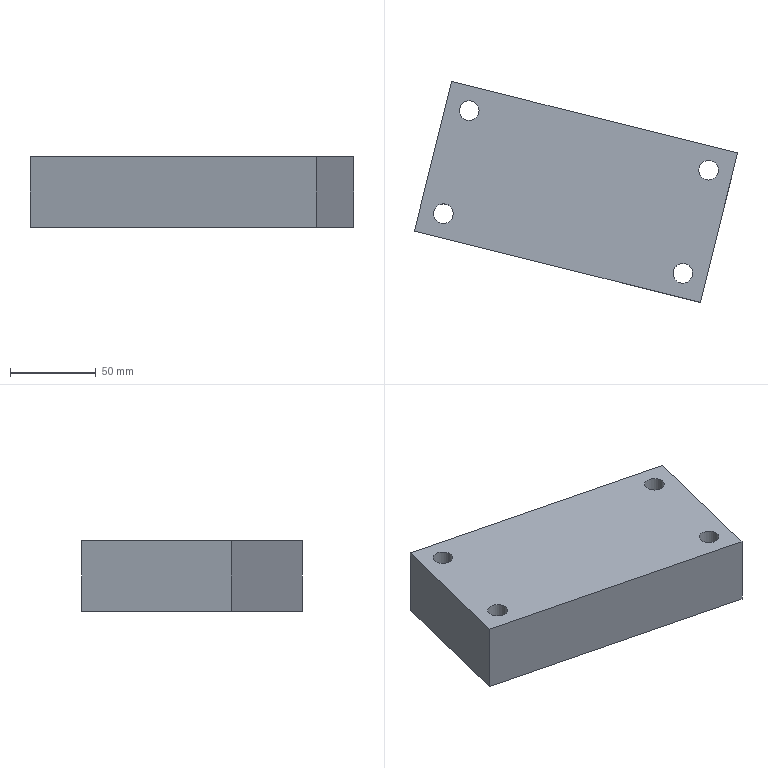Part | NX | features solid 2 | 1 solid | 18 faces | box 188.664 x 128.937 x 41 mm | volume 609814 mm3 | plane 10 | cylinder 8 | commonest cylinder face diameters 11.5 x4 18 x4
STEP:
#1=CARTESIAN_POINT('',(1088.08,30.743,73.));
#2=VERTEX_POINT('',#1);
#3=CARTESIAN_POINT('',(1086.688,25.164,73.));
#4=DIRECTION('',(0.,0.,-1.));
#5=DIRECTION('',(0.2419,0.9703,0.));
#6=AXIS2_PLACEMENT_3D('',#3,#4,#5);
#7=CIRCLE('',#6,5.75);
#8=EDGE_CURVE('',#2,#2,#7,.T.);
#9=ORIENTED_EDGE('',*,*,#8,.F.);
#10=EDGE_LOOP('',(#9));
#11=FACE_BOUND('',#10,.T.);
#12=CARTESIAN_POINT('',(1088.866,33.896,73.));
#13=VERTEX_POINT('',#12);
#14=CARTESIAN_POINT('',(1086.688,25.164,73.));
#15=DIRECTION('',(0.,0.,-1.));
#16=DIRECTION('',(0.2419,0.9703,0.));
#17=AXIS2_PLACEMENT_3D('',#14,#15,#16);
#18=CIRCLE('',#17,9.);
#19=EDGE_CURVE('',#13,#13,#18,.T.);
#20=ORIENTED_EDGE('',*,*,#19,.T.);
#21=EDGE_LOOP('',(#20));
#22=FACE_BOUND('',#21,.T.);
#23=CARTESIAN_POINT('',(1086.688,25.164,73.));
#24=DIRECTION('',(0.,0.,1.));
#25=DIRECTION('',(-0.2419,-0.9703,0.));
#26=AXIS2_PLACEMENT_3D('',#23,#24,#25);
#27=PLANE('',#26);
#28=ADVANCED_FACE('',(#11,#22),#27,.F.);
#29=CARTESIAN_POINT('',(1103.079,90.901,73.));
#30=VERTEX_POINT('',#29);
#31=CARTESIAN_POINT('',(1101.688,85.322,73.));
#32=DIRECTION('',(0.,0.,-1.));
#33=DIRECTION('',(0.2419,0.9703,0.));
#34=AXIS2_PLACEMENT_3D('',#31,#32,#33);
#35=CIRCLE('',#34,5.75);
#36=EDGE_CURVE('',#30,#30,#35,.T.);
#37=ORIENTED_EDGE('',*,*,#36,.F.);
#38=EDGE_LOOP('',(#37));
#39=FACE_BOUND('',#38,.T.);
#40=CARTESIAN_POINT('',(1103.865,94.055,73.));
#41=VERTEX_POINT('',#40);
#42=CARTESIAN_POINT('',(1101.688,85.322,73.));
#43=DIRECTION('',(0.,0.,-1.));
#44=DIRECTION('',(0.2419,0.9703,0.));
#45=AXIS2_PLACEMENT_3D('',#42,#43,#44);
#46=CIRCLE('',#45,9.);
#47=EDGE_CURVE('',#41,#41,#46,.T.);
#48=ORIENTED_EDGE('',*,*,#47,.T.);
#49=EDGE_LOOP('',(#48));
#50=FACE_BOUND('',#49,.T.);
#51=CARTESIAN_POINT('',(1101.688,85.322,73.));
#52=DIRECTION('',(0.,0.,1.));
#53=DIRECTION('',(-0.2419,-0.9703,0.));
#54=AXIS2_PLACEMENT_3D('',#51,#52,#53);
#55=PLANE('',#54);
#56=ADVANCED_FACE('',(#39,#50),#55,.F.);
#57=CARTESIAN_POINT('',(948.357,65.58,73.));
#58=VERTEX_POINT('',#57);
#59=CARTESIAN_POINT('',(946.966,60.,73.));
#60=DIRECTION('',(0.,0.,-1.));
#61=DIRECTION('',(0.2419,0.9703,0.));
#62=AXIS2_PLACEMENT_3D('',#59,#60,#61);
#63=CIRCLE('',#62,5.75);
#64=EDGE_CURVE('',#58,#58,#63,.T.);
#65=ORIENTED_EDGE('',*,*,#64,.F.);
#66=EDGE_LOOP('',(#65));
#67=FACE_BOUND('',#66,.T.);
#68=CARTESIAN_POINT('',(949.143,68.733,73.));
#69=VERTEX_POINT('',#68);
#70=CARTESIAN_POINT('',(946.966,60.,73.));
#71=DIRECTION('',(0.,0.,-1.));
#72=DIRECTION('',(0.2419,0.9703,0.));
#73=AXIS2_PLACEMENT_3D('',#70,#71,#72);
#74=CIRCLE('',#73,9.);
#75=EDGE_CURVE('',#69,#69,#74,.T.);
#76=ORIENTED_EDGE('',*,*,#75,.T.);
#77=EDGE_LOOP('',(#76));
#78=FACE_BOUND('',#77,.T.);
#79=CARTESIAN_POINT('',(946.966,60.,73.));
#80=DIRECTION('',(0.,0.,1.));
#81=DIRECTION('',(-0.2419,-0.9703,0.));
#82=AXIS2_PLACEMENT_3D('',#79,#80,#81);
#83=PLANE('',#82);
#84=ADVANCED_FACE('',(#67,#78),#83,.F.);
#85=ORIENTED_EDGE('',*,*,#47,.F.);
#86=EDGE_LOOP('',(#85));
#87=FACE_BOUND('',#86,.T.);
#88=CARTESIAN_POINT('',(1103.865,94.055,60.));
#89=VERTEX_POINT('',#88);
#90=CARTESIAN_POINT('',(1101.688,85.322,60.));
#91=DIRECTION('',(0.,0.,-1.));
#92=DIRECTION('',(0.2419,0.9703,0.));
#93=AXIS2_PLACEMENT_3D('',#90,#91,#92);
#94=CIRCLE('',#93,9.);
#95=EDGE_CURVE('',#89,#89,#94,.T.);
#96=ORIENTED_EDGE('',*,*,#95,.T.);
#97=EDGE_LOOP('',(#96));
#98=FACE_BOUND('',#97,.T.);
#99=CARTESIAN_POINT('',(1101.688,85.322,60.));
#100=DIRECTION('',(0.,0.,1.));
#101=DIRECTION('',(-0.2419,-0.9703,0.));
#102=AXIS2_PLACEMENT_3D('',#99,#100,#101);
#103=CYLINDRICAL_SURFACE('',#102,9.);
#104=ADVANCED_FACE('',(#87,#98),#103,.F.);
#105=ORIENTED_EDGE('',*,*,#75,.F.);
#106=EDGE_LOOP('',(#105));
#107=FACE_BOUND('',#106,.T.);
#108=CARTESIAN_POINT('',(949.143,68.733,60.));
#109=VERTEX_POINT('',#108);
#110=CARTESIAN_POINT('',(946.966,60.,60.));
#111=DIRECTION('',(0.,0.,-1.));
#112=DIRECTION('',(0.2419,0.9703,0.));
#113=AXIS2_PLACEMENT_3D('',#110,#111,#112);
#114=CIRCLE('',#113,9.);
#115=EDGE_CURVE('',#109,#109,#114,.T.);
#116=ORIENTED_EDGE('',*,*,#115,.T.);
#117=EDGE_LOOP('',(#116));
#118=FACE_BOUND('',#117,.T.);
#119=CARTESIAN_POINT('',(946.966,60.,60.));
#120=DIRECTION('',(0.,0.,1.));
#121=DIRECTION('',(-0.2419,-0.9703,0.));
#122=AXIS2_PLACEMENT_3D('',#119,#120,#121);
#123=CYLINDRICAL_SURFACE('',#122,9.);
#124=ADVANCED_FACE('',(#107,#118),#123,.F.);
#125=CARTESIAN_POINT('',(1118.659,95.519,101.));
#126=VERTEX_POINT('',#125);
#127=CARTESIAN_POINT('',(951.768,137.13,101.));
#128=VERTEX_POINT('',#127);
#129=CARTESIAN_POINT('',(1045.886,113.663,101.));
#130=DIRECTION('',(-0.9703,0.2419,0.));
#131=VECTOR('',#130,1000.);
#132=LINE('',#129,#131);
#133=EDGE_CURVE('',#126,#128,#132,.T.);
#134=ORIENTED_EDGE('',*,*,#133,.F.);
#135=CARTESIAN_POINT('',(1118.659,95.519,60.));
#136=VERTEX_POINT('',#135);
#137=CARTESIAN_POINT('',(1118.659,95.519,-25.));
#138=DIRECTION('',(0.,0.,1.));
#139=VECTOR('',#138,1000.);
#140=LINE('',#137,#139);
#141=EDGE_CURVE('',#136,#126,#140,.T.);
#142=ORIENTED_EDGE('',*,*,#141,.F.);
#143=CARTESIAN_POINT('',(951.768,137.13,60.));
#144=VERTEX_POINT('',#143);
#145=CARTESIAN_POINT('',(1045.886,113.663,60.));
#146=DIRECTION('',(0.9703,-0.2419,0.));
#147=VECTOR('',#146,1000.);
#148=LINE('',#145,#147);
#149=EDGE_CURVE('',#144,#136,#148,.T.);
#150=ORIENTED_EDGE('',*,*,#149,.F.);
#151=CARTESIAN_POINT('',(951.768,137.13,-25.));
#152=DIRECTION('',(0.,0.,1.));
#153=VECTOR('',#152,1000.);
#154=LINE('',#151,#153);
#155=EDGE_CURVE('',#144,#128,#154,.T.);
#156=ORIENTED_EDGE('',*,*,#155,.T.);
#157=EDGE_LOOP('',(#134,#142,#150,#156));
#158=FACE_BOUND('',#157,.T.);
#159=CARTESIAN_POINT('',(1045.886,113.663,-25.));
#160=DIRECTION('',(0.2419,0.9703,0.));
#161=DIRECTION('',(0.,0.,1.));
#162=AXIS2_PLACEMENT_3D('',#159,#160,#161);
#163=PLANE('',#162);
#164=ADVANCED_FACE('',(#158),#163,.T.);
#165=CARTESIAN_POINT('',(1096.886,8.193,60.));
#166=VERTEX_POINT('',#165);
#167=CARTESIAN_POINT('',(1096.886,8.193,101.));
#168=VERTEX_POINT('',#167);
#169=CARTESIAN_POINT('',(1096.886,8.193,-25.));
#170=DIRECTION('',(0.,0.,1.));
#171=VECTOR('',#170,1000.);
#172=LINE('',#169,#171);
#173=EDGE_CURVE('',#166,#168,#172,.T.);
#174=ORIENTED_EDGE('',*,*,#173,.F.);
#175=CARTESIAN_POINT('',(1107.772,51.856,60.));
#176=DIRECTION('',(-0.2419,-0.9703,0.));
#177=VECTOR('',#176,1000.);
#178=LINE('',#175,#177);
#179=EDGE_CURVE('',#136,#166,#178,.T.);
#180=ORIENTED_EDGE('',*,*,#179,.F.);
#181=ORIENTED_EDGE('',*,*,#141,.T.);
#182=CARTESIAN_POINT('',(1107.772,51.856,101.));
#183=DIRECTION('',(0.2419,0.9703,0.));
#184=VECTOR('',#183,1000.);
#185=LINE('',#182,#184);
#186=EDGE_CURVE('',#168,#126,#185,.T.);
#187=ORIENTED_EDGE('',*,*,#186,.F.);
#188=EDGE_LOOP('',(#174,#180,#181,#187));
#189=FACE_BOUND('',#188,.T.);
#190=CARTESIAN_POINT('',(1107.772,51.856,-25.));
#191=DIRECTION('',(0.9703,-0.2419,0.));
#192=DIRECTION('',(0.,0.,-1.));
#193=AXIS2_PLACEMENT_3D('',#190,#191,#192);
#194=PLANE('',#193);
#195=ADVANCED_FACE('',(#189),#194,.T.);
#196=CARTESIAN_POINT('',(929.995,49.803,60.));
#197=VERTEX_POINT('',#196);
#198=CARTESIAN_POINT('',(929.995,49.803,101.));
#199=VERTEX_POINT('',#198);
#200=CARTESIAN_POINT('',(929.995,49.803,-25.));
#201=DIRECTION('',(0.,0.,1.));
#202=VECTOR('',#201,1000.);
#203=LINE('',#200,#202);
#204=EDGE_CURVE('',#197,#199,#203,.T.);
#205=ORIENTED_EDGE('',*,*,#204,.F.);
#206=CARTESIAN_POINT('',(1024.114,26.337,60.));
#207=DIRECTION('',(-0.9703,0.2419,0.));
#208=VECTOR('',#207,1000.);
#209=LINE('',#206,#208);
#210=EDGE_CURVE('',#166,#197,#209,.T.);
#211=ORIENTED_EDGE('',*,*,#210,.F.);
#212=ORIENTED_EDGE('',*,*,#173,.T.);
#213=CARTESIAN_POINT('',(1024.114,26.337,101.));
#214=DIRECTION('',(0.9703,-0.2419,0.));
#215=VECTOR('',#214,1000.);
#216=LINE('',#213,#215);
#217=EDGE_CURVE('',#199,#168,#216,.T.);
#218=ORIENTED_EDGE('',*,*,#217,.F.);
#219=EDGE_LOOP('',(#205,#211,#212,#218));
#220=FACE_BOUND('',#219,.T.);
#221=CARTESIAN_POINT('',(1024.114,26.337,-25.));
#222=DIRECTION('',(-0.2419,-0.9703,0.));
#223=DIRECTION('',(0.,0.,-1.));
#224=AXIS2_PLACEMENT_3D('',#221,#222,#223);
#225=PLANE('',#224);
#226=ADVANCED_FACE('',(#220),#225,.T.);
#227=CARTESIAN_POINT('',(940.881,93.466,60.));
#228=DIRECTION('',(0.2419,0.9703,0.));
#229=VECTOR('',#228,1000.);
#230=LINE('',#227,#229);
#231=EDGE_CURVE('',#197,#144,#230,.T.);
#232=ORIENTED_EDGE('',*,*,#231,.F.);
#233=ORIENTED_EDGE('',*,*,#204,.T.);
#234=CARTESIAN_POINT('',(940.881,93.466,101.));
#235=DIRECTION('',(-0.2419,-0.9703,0.));
#236=VECTOR('',#235,1000.);
#237=LINE('',#234,#236);
#238=EDGE_CURVE('',#128,#199,#237,.T.);
#239=ORIENTED_EDGE('',*,*,#238,.F.);
#240=ORIENTED_EDGE('',*,*,#155,.F.);
#241=EDGE_LOOP('',(#232,#233,#239,#240));
#242=FACE_BOUND('',#241,.T.);
#243=CARTESIAN_POINT('',(940.881,93.466,-25.));
#244=DIRECTION('',(-0.9703,0.2419,0.));
#245=DIRECTION('',(0.,0.,1.));
#246=AXIS2_PLACEMENT_3D('',#243,#244,#245);
#247=PLANE('',#246);
#248=ADVANCED_FACE('',(#242),#247,.T.);
#249=CARTESIAN_POINT('',(1088.08,30.743,101.));
#250=VERTEX_POINT('',#249);
#251=CARTESIAN_POINT('',(1086.688,25.164,101.));
#252=DIRECTION('',(0.,0.,-1.));
#253=DIRECTION('',(0.2419,0.9703,0.));
#254=AXIS2_PLACEMENT_3D('',#251,#252,#253);
#255=CIRCLE('',#254,5.75);
#256=EDGE_CURVE('',#250,#250,#255,.T.);
#257=ORIENTED_EDGE('',*,*,#256,.F.);
#258=EDGE_LOOP('',(#257));
#259=FACE_BOUND('',#258,.T.);
#260=ORIENTED_EDGE('',*,*,#8,.T.);
#261=EDGE_LOOP('',(#260));
#262=FACE_BOUND('',#261,.T.);
#263=CARTESIAN_POINT('',(1086.688,25.164,55.));
#264=DIRECTION('',(0.,0.,1.));
#265=DIRECTION('',(-0.2419,-0.9703,0.));
#266=AXIS2_PLACEMENT_3D('',#263,#264,#265);
#267=CYLINDRICAL_SURFACE('',#266,5.75);
#268=ADVANCED_FACE('',(#259,#262),#267,.F.);
#269=CARTESIAN_POINT('',(1103.079,90.901,101.));
#270=VERTEX_POINT('',#269);
#271=CARTESIAN_POINT('',(1101.688,85.322,101.));
#272=DIRECTION('',(0.,0.,-1.));
#273=DIRECTION('',(0.2419,0.9703,0.));
#274=AXIS2_PLACEMENT_3D('',#271,#272,#273);
#275=CIRCLE('',#274,5.75);
#276=EDGE_CURVE('',#270,#270,#275,.T.);
#277=ORIENTED_EDGE('',*,*,#276,.F.);
#278=EDGE_LOOP('',(#277));
#279=FACE_BOUND('',#278,.T.);
#280=ORIENTED_EDGE('',*,*,#36,.T.);
#281=EDGE_LOOP('',(#280));
#282=FACE_BOUND('',#281,.T.);
#283=CARTESIAN_POINT('',(1101.688,85.322,55.));
#284=DIRECTION('',(0.,0.,1.));
#285=DIRECTION('',(-0.2419,-0.9703,0.));
#286=AXIS2_PLACEMENT_3D('',#283,#284,#285);
#287=CYLINDRICAL_SURFACE('',#286,5.75);
#288=ADVANCED_FACE('',(#279,#282),#287,.F.);
#289=CARTESIAN_POINT('',(948.357,65.58,101.));
#290=VERTEX_POINT('',#289);
#291=CARTESIAN_POINT('',(946.966,60.,101.));
#292=DIRECTION('',(0.,0.,-1.));
#293=DIRECTION('',(0.2419,0.9703,0.));
#294=AXIS2_PLACEMENT_3D('',#291,#292,#293);
#295=CIRCLE('',#294,5.75);
#296=EDGE_CURVE('',#290,#290,#295,.T.);
#297=ORIENTED_EDGE('',*,*,#296,.F.);
#298=EDGE_LOOP('',(#297));
#299=FACE_BOUND('',#298,.T.);
#300=ORIENTED_EDGE('',*,*,#64,.T.);
#301=EDGE_LOOP('',(#300));
#302=FACE_BOUND('',#301,.T.);
#303=CARTESIAN_POINT('',(946.966,60.,55.));
#304=DIRECTION('',(0.,0.,1.));
#305=DIRECTION('',(-0.2419,-0.9703,0.));
#306=AXIS2_PLACEMENT_3D('',#303,#304,#305);
#307=CYLINDRICAL_SURFACE('',#306,5.75);
#308=ADVANCED_FACE('',(#299,#302),#307,.F.);
#309=CARTESIAN_POINT('',(967.715,120.159,101.));
#310=VERTEX_POINT('',#309);
#311=CARTESIAN_POINT('',(961.965,120.159,101.));
#312=DIRECTION('',(0.,0.,1.));
#313=DIRECTION('',(1.,0.,0.));
#314=AXIS2_PLACEMENT_3D('',#311,#312,#313);
#315=CIRCLE('',#314,5.75);
#316=EDGE_CURVE('',#310,#310,#315,.T.);
#317=ORIENTED_EDGE('',*,*,#316,.F.);
#318=EDGE_LOOP('',(#317));
#319=FACE_BOUND('',#318,.T.);
#320=ORIENTED_EDGE('',*,*,#296,.T.);
#321=EDGE_LOOP('',(#320));
#322=FACE_BOUND('',#321,.T.);
#323=ORIENTED_EDGE('',*,*,#276,.T.);
#324=EDGE_LOOP('',(#323));
#325=FACE_BOUND('',#324,.T.);
#326=ORIENTED_EDGE('',*,*,#256,.T.);
#327=EDGE_LOOP('',(#326));
#328=FACE_BOUND('',#327,.T.);
#329=ORIENTED_EDGE('',*,*,#238,.T.);
#330=ORIENTED_EDGE('',*,*,#217,.T.);
#331=ORIENTED_EDGE('',*,*,#186,.T.);
#332=ORIENTED_EDGE('',*,*,#133,.T.);
#333=EDGE_LOOP('',(#329,#330,#331,#332));
#334=FACE_BOUND('',#333,.T.);
#335=CARTESIAN_POINT('',(1333.794,-872.79,101.));
#336=DIRECTION('',(0.,0.,1.));
#337=DIRECTION('',(-0.2419,-0.9703,0.));
#338=AXIS2_PLACEMENT_3D('',#335,#336,#337);
#339=PLANE('',#338);
#340=ADVANCED_FACE('',(#319,#322,#325,#328,#334),#339,.T.);
#341=ORIENTED_EDGE('',*,*,#19,.F.);
#342=EDGE_LOOP('',(#341));
#343=FACE_BOUND('',#342,.T.);
#344=CARTESIAN_POINT('',(1088.866,33.896,60.));
#345=VERTEX_POINT('',#344);
#346=CARTESIAN_POINT('',(1086.688,25.164,60.));
#347=DIRECTION('',(0.,0.,-1.));
#348=DIRECTION('',(0.2419,0.9703,0.));
#349=AXIS2_PLACEMENT_3D('',#346,#347,#348);
#350=CIRCLE('',#349,9.);
#351=EDGE_CURVE('',#345,#345,#350,.T.);
#352=ORIENTED_EDGE('',*,*,#351,.T.);
#353=EDGE_LOOP('',(#352));
#354=FACE_BOUND('',#353,.T.);
#355=CARTESIAN_POINT('',(1086.688,25.164,60.));
#356=DIRECTION('',(0.,0.,1.));
#357=DIRECTION('',(-0.2419,-0.9703,0.));
#358=AXIS2_PLACEMENT_3D('',#355,#356,#357);
#359=CYLINDRICAL_SURFACE('',#358,9.);
#360=ADVANCED_FACE('',(#343,#354),#359,.F.);
#361=CARTESIAN_POINT('',(970.965,120.159,60.));
#362=VERTEX_POINT('',#361);
#363=CARTESIAN_POINT('',(961.965,120.159,60.));
#364=DIRECTION('',(0.,0.,-1.));
#365=DIRECTION('',(1.,0.,0.));
#366=AXIS2_PLACEMENT_3D('',#363,#364,#365);
#367=CIRCLE('',#366,9.);
#368=EDGE_CURVE('',#362,#362,#367,.T.);
#369=ORIENTED_EDGE('',*,*,#368,.F.);
#370=EDGE_LOOP('',(#369));
#371=FACE_BOUND('',#370,.T.);
#372=ORIENTED_EDGE('',*,*,#351,.F.);
#373=EDGE_LOOP('',(#372));
#374=FACE_BOUND('',#373,.T.);
#375=ORIENTED_EDGE('',*,*,#115,.F.);
#376=EDGE_LOOP('',(#375));
#377=FACE_BOUND('',#376,.T.);
#378=ORIENTED_EDGE('',*,*,#95,.F.);
#379=EDGE_LOOP('',(#378));
#380=FACE_BOUND('',#379,.T.);
#381=ORIENTED_EDGE('',*,*,#149,.T.);
#382=ORIENTED_EDGE('',*,*,#179,.T.);
#383=ORIENTED_EDGE('',*,*,#210,.T.);
#384=ORIENTED_EDGE('',*,*,#231,.T.);
#385=EDGE_LOOP('',(#381,#382,#383,#384));
#386=FACE_BOUND('',#385,.T.);
#387=CARTESIAN_POINT('',(1637.628,1143.602,60.));
#388=DIRECTION('',(0.,0.,1.));
#389=DIRECTION('',(-0.2419,-0.9703,0.));
#390=AXIS2_PLACEMENT_3D('',#387,#388,#389);
#391=PLANE('',#390);
#392=ADVANCED_FACE('',(#371,#374,#377,#380,#386),#391,.F.);
#393=CARTESIAN_POINT('',(963.356,125.738,73.));
#394=VERTEX_POINT('',#393);
#395=CARTESIAN_POINT('',(961.965,120.159,73.));
#396=DIRECTION('',(0.,0.,-1.));
#397=DIRECTION('',(0.2419,0.9703,0.));
#398=AXIS2_PLACEMENT_3D('',#395,#396,#397);
#399=CIRCLE('',#398,5.75);
#400=EDGE_CURVE('',#394,#394,#399,.T.);
#401=ORIENTED_EDGE('',*,*,#400,.F.);
#402=EDGE_LOOP('',(#401));
#403=FACE_BOUND('',#402,.T.);
#404=CARTESIAN_POINT('',(964.142,128.891,73.));
#405=VERTEX_POINT('',#404);
#406=CARTESIAN_POINT('',(961.965,120.159,73.));
#407=DIRECTION('',(0.,0.,-1.));
#408=DIRECTION('',(0.2419,0.9703,0.));
#409=AXIS2_PLACEMENT_3D('',#406,#407,#408);
#410=CIRCLE('',#409,9.);
#411=EDGE_CURVE('',#405,#405,#410,.T.);
#412=ORIENTED_EDGE('',*,*,#411,.T.);
#413=EDGE_LOOP('',(#412));
#414=FACE_BOUND('',#413,.T.);
#415=CARTESIAN_POINT('',(961.965,120.159,73.));
#416=DIRECTION('',(0.,0.,1.));
#417=DIRECTION('',(-0.2419,-0.9703,0.));
#418=AXIS2_PLACEMENT_3D('',#415,#416,#417);
#419=PLANE('',#418);
#420=ADVANCED_FACE('',(#403,#414),#419,.F.);
#421=ORIENTED_EDGE('',*,*,#316,.T.);
#422=EDGE_LOOP('',(#421));
#423=FACE_BOUND('',#422,.T.);
#424=ORIENTED_EDGE('',*,*,#400,.T.);
#425=EDGE_LOOP('',(#424));
#426=FACE_BOUND('',#425,.T.);
#427=CARTESIAN_POINT('',(961.965,120.159,55.));
#428=DIRECTION('',(0.,0.,1.));
#429=DIRECTION('',(-0.2419,-0.9703,0.));
#430=AXIS2_PLACEMENT_3D('',#427,#428,#429);
#431=CYLINDRICAL_SURFACE('',#430,5.75);
#432=ADVANCED_FACE('',(#423,#426),#431,.F.);
#433=ORIENTED_EDGE('',*,*,#411,.F.);
#434=EDGE_LOOP('',(#433));
#435=FACE_BOUND('',#434,.T.);
#436=ORIENTED_EDGE('',*,*,#368,.T.);
#437=EDGE_LOOP('',(#436));
#438=FACE_BOUND('',#437,.T.);
#439=CARTESIAN_POINT('',(961.965,120.159,60.));
#440=DIRECTION('',(0.,0.,1.));
#441=DIRECTION('',(-0.2419,-0.9703,0.));
#442=AXIS2_PLACEMENT_3D('',#439,#440,#441);
#443=CYLINDRICAL_SURFACE('',#442,9.);
#444=ADVANCED_FACE('',(#435,#438),#443,.F.);
#445=CLOSED_SHELL('',(#28,#56,#84,#104,#124,#164,#195,#226,#248,#268,#288,#308,#340,#360,#392,#420,#432,#444));
#446=MANIFOLD_SOLID_BREP('',#445);
#447=(LENGTH_UNIT()NAMED_UNIT(*)SI_UNIT(.MILLI.,.METRE.));
#448=UNCERTAINTY_MEASURE_WITH_UNIT(LENGTH_MEASURE(0.00001),#447,'','');
#449=(NAMED_UNIT(*)PLANE_ANGLE_UNIT()SI_UNIT($,.RADIAN.));
#450=(NAMED_UNIT(*)SI_UNIT($,.STERADIAN.)SOLID_ANGLE_UNIT());
#451=(GEOMETRIC_REPRESENTATION_CONTEXT(3)GLOBAL_UNCERTAINTY_ASSIGNED_CONTEXT((#448))GLOBAL_UNIT_ASSIGNED_CONTEXT((#447,#449,#450))REPRESENTATION_CONTEXT('',''));
#452=ADVANCED_BREP_SHAPE_REPRESENTATION('',(#446),#451);